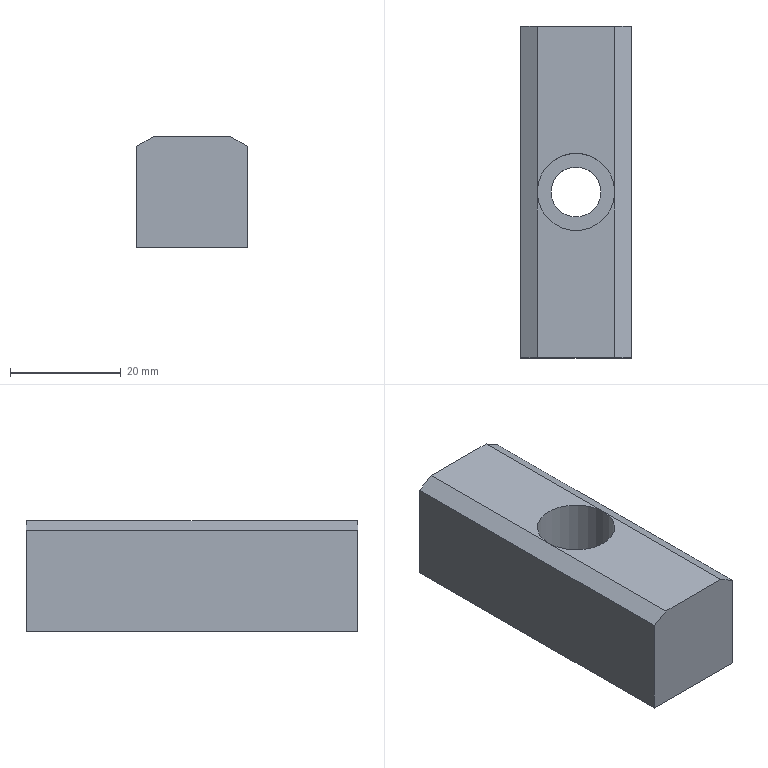Part | NX | features solid 2 | 1 solid | 12 faces | box 20 x 60 x 20 mm | volume 21513 mm3 | plane 10 | cylinder 2 | commonest cylinder face diameters 9 x1 14 x1
STEP:
#1=CARTESIAN_POINT('',(-7.,-353.,-45.));
#2=VERTEX_POINT('',#1);
#3=CARTESIAN_POINT('',(7.,-353.,-45.));
#4=VERTEX_POINT('',#3);
#5=CARTESIAN_POINT('',(-10.,-353.,-45.));
#6=DIRECTION('',(1.,0.,0.));
#7=VECTOR('',#6,1000.);
#8=LINE('',#5,#7);
#9=EDGE_CURVE('',#2,#4,#8,.T.);
#10=ORIENTED_EDGE('',*,*,#9,.T.);
#11=CARTESIAN_POINT('',(7.,-323.,-45.));
#12=VERTEX_POINT('',#11);
#13=CARTESIAN_POINT('',(7.,-353.,-45.));
#14=DIRECTION('',(0.,-1.,0.));
#15=VECTOR('',#14,1000.);
#16=LINE('',#13,#15);
#17=EDGE_CURVE('',#4,#12,#16,.F.);
#18=ORIENTED_EDGE('',*,*,#17,.T.);
#19=CARTESIAN_POINT('',(-7.,-323.,-45.));
#20=VERTEX_POINT('',#19);
#21=CARTESIAN_POINT('',(0.,-323.,-45.));
#22=DIRECTION('',(0.,0.,-1.));
#23=DIRECTION('',(-1.,0.,0.));
#24=AXIS2_PLACEMENT_3D('',#21,#22,#23);
#25=CIRCLE('',#24,7.);
#26=EDGE_CURVE('',#12,#20,#25,.T.);
#27=ORIENTED_EDGE('',*,*,#26,.T.);
#28=CARTESIAN_POINT('',(-7.,-353.,-45.));
#29=DIRECTION('',(0.,1.,0.));
#30=VECTOR('',#29,1000.);
#31=LINE('',#28,#30);
#32=EDGE_CURVE('',#20,#2,#31,.F.);
#33=ORIENTED_EDGE('',*,*,#32,.T.);
#34=EDGE_LOOP('',(#10,#18,#27,#33));
#35=FACE_BOUND('',#34,.T.);
#36=CARTESIAN_POINT('',(-10.,-353.,-45.));
#37=DIRECTION('',(0.,0.,-1.));
#38=DIRECTION('',(0.,1.,0.));
#39=AXIS2_PLACEMENT_3D('',#36,#37,#38);
#40=PLANE('',#39);
#41=ADVANCED_FACE('',(#35),#40,.F.);
#42=CARTESIAN_POINT('',(-4.5,-323.,-65.));
#43=VERTEX_POINT('',#42);
#44=CARTESIAN_POINT('',(0.,-323.,-65.));
#45=DIRECTION('',(0.,0.,-1.));
#46=DIRECTION('',(-1.,0.,0.));
#47=AXIS2_PLACEMENT_3D('',#44,#45,#46);
#48=CIRCLE('',#47,4.5);
#49=EDGE_CURVE('',#43,#43,#48,.T.);
#50=ORIENTED_EDGE('',*,*,#49,.F.);
#51=EDGE_LOOP('',(#50));
#52=FACE_BOUND('',#51,.T.);
#53=CARTESIAN_POINT('',(-10.,-353.,-65.));
#54=VERTEX_POINT('',#53);
#55=CARTESIAN_POINT('',(10.,-353.,-65.));
#56=VERTEX_POINT('',#55);
#57=CARTESIAN_POINT('',(-10.,-353.,-65.));
#58=DIRECTION('',(1.,0.,0.));
#59=VECTOR('',#58,1000.);
#60=LINE('',#57,#59);
#61=EDGE_CURVE('',#54,#56,#60,.T.);
#62=ORIENTED_EDGE('',*,*,#61,.F.);
#63=CARTESIAN_POINT('',(-10.,-293.,-65.));
#64=VERTEX_POINT('',#63);
#65=CARTESIAN_POINT('',(-10.,-353.,-65.));
#66=DIRECTION('',(0.,1.,0.));
#67=VECTOR('',#66,1000.);
#68=LINE('',#65,#67);
#69=EDGE_CURVE('',#54,#64,#68,.T.);
#70=ORIENTED_EDGE('',*,*,#69,.T.);
#71=CARTESIAN_POINT('',(10.,-293.,-65.));
#72=VERTEX_POINT('',#71);
#73=CARTESIAN_POINT('',(-10.,-293.,-65.));
#74=DIRECTION('',(1.,0.,0.));
#75=VECTOR('',#74,1000.);
#76=LINE('',#73,#75);
#77=EDGE_CURVE('',#64,#72,#76,.T.);
#78=ORIENTED_EDGE('',*,*,#77,.T.);
#79=CARTESIAN_POINT('',(10.,-353.,-65.));
#80=DIRECTION('',(0.,1.,0.));
#81=VECTOR('',#80,1000.);
#82=LINE('',#79,#81);
#83=EDGE_CURVE('',#56,#72,#82,.T.);
#84=ORIENTED_EDGE('',*,*,#83,.F.);
#85=EDGE_LOOP('',(#62,#70,#78,#84));
#86=FACE_BOUND('',#85,.T.);
#87=CARTESIAN_POINT('',(-10.,-353.,-65.));
#88=DIRECTION('',(0.,0.,-1.));
#89=DIRECTION('',(0.,1.,0.));
#90=AXIS2_PLACEMENT_3D('',#87,#88,#89);
#91=PLANE('',#90);
#92=ADVANCED_FACE('',(#52,#86),#91,.T.);
#93=CARTESIAN_POINT('',(-7.,-293.,-45.));
#94=VERTEX_POINT('',#93);
#95=CARTESIAN_POINT('',(7.,-293.,-45.));
#96=VERTEX_POINT('',#95);
#97=CARTESIAN_POINT('',(-10.,-293.,-45.));
#98=DIRECTION('',(1.,0.,0.));
#99=VECTOR('',#98,1000.);
#100=LINE('',#97,#99);
#101=EDGE_CURVE('',#94,#96,#100,.T.);
#102=ORIENTED_EDGE('',*,*,#101,.T.);
#103=CARTESIAN_POINT('',(10.,-293.,-46.732));
#104=VERTEX_POINT('',#103);
#105=CARTESIAN_POINT('',(2.91,-293.,-42.639));
#106=DIRECTION('',(0.866,0.,-0.5));
#107=VECTOR('',#106,1000.);
#108=LINE('',#105,#107);
#109=EDGE_CURVE('',#96,#104,#108,.T.);
#110=ORIENTED_EDGE('',*,*,#109,.T.);
#111=CARTESIAN_POINT('',(10.,-293.,-65.));
#112=DIRECTION('',(0.,0.,-1.));
#113=VECTOR('',#112,1000.);
#114=LINE('',#111,#113);
#115=EDGE_CURVE('',#72,#104,#114,.F.);
#116=ORIENTED_EDGE('',*,*,#115,.F.);
#117=ORIENTED_EDGE('',*,*,#77,.F.);
#118=CARTESIAN_POINT('',(-10.,-293.,-46.732));
#119=VERTEX_POINT('',#118);
#120=CARTESIAN_POINT('',(-10.,-293.,-65.));
#121=DIRECTION('',(0.,0.,1.));
#122=VECTOR('',#121,1000.);
#123=LINE('',#120,#122);
#124=EDGE_CURVE('',#64,#119,#123,.T.);
#125=ORIENTED_EDGE('',*,*,#124,.T.);
#126=CARTESIAN_POINT('',(-17.91,-293.,-51.299));
#127=DIRECTION('',(-0.866,0.,-0.5));
#128=VECTOR('',#127,1000.);
#129=LINE('',#126,#128);
#130=EDGE_CURVE('',#119,#94,#129,.F.);
#131=ORIENTED_EDGE('',*,*,#130,.T.);
#132=EDGE_LOOP('',(#102,#110,#116,#117,#125,#131));
#133=FACE_BOUND('',#132,.T.);
#134=CARTESIAN_POINT('',(-10.,-293.,-65.));
#135=DIRECTION('',(0.,1.,0.));
#136=DIRECTION('',(0.,0.,1.));
#137=AXIS2_PLACEMENT_3D('',#134,#135,#136);
#138=PLANE('',#137);
#139=ADVANCED_FACE('',(#133),#138,.T.);
#140=CARTESIAN_POINT('',(0.,-323.,-45.));
#141=DIRECTION('',(0.,0.,-1.));
#142=DIRECTION('',(-1.,0.,0.));
#143=AXIS2_PLACEMENT_3D('',#140,#141,#142);
#144=CIRCLE('',#143,7.);
#145=EDGE_CURVE('',#20,#12,#144,.T.);
#146=ORIENTED_EDGE('',*,*,#145,.T.);
#147=CARTESIAN_POINT('',(7.,-353.,-45.));
#148=DIRECTION('',(0.,-1.,0.));
#149=VECTOR('',#148,1000.);
#150=LINE('',#147,#149);
#151=EDGE_CURVE('',#12,#96,#150,.F.);
#152=ORIENTED_EDGE('',*,*,#151,.T.);
#153=ORIENTED_EDGE('',*,*,#101,.F.);
#154=CARTESIAN_POINT('',(-7.,-353.,-45.));
#155=DIRECTION('',(0.,1.,0.));
#156=VECTOR('',#155,1000.);
#157=LINE('',#154,#156);
#158=EDGE_CURVE('',#94,#20,#157,.F.);
#159=ORIENTED_EDGE('',*,*,#158,.T.);
#160=EDGE_LOOP('',(#146,#152,#153,#159));
#161=FACE_BOUND('',#160,.T.);
#162=CARTESIAN_POINT('',(-10.,-353.,-45.));
#163=DIRECTION('',(0.,0.,-1.));
#164=DIRECTION('',(0.,1.,0.));
#165=AXIS2_PLACEMENT_3D('',#162,#163,#164);
#166=PLANE('',#165);
#167=ADVANCED_FACE('',(#161),#166,.F.);
#168=ORIENTED_EDGE('',*,*,#115,.T.);
#169=CARTESIAN_POINT('',(10.,-353.,-46.732));
#170=VERTEX_POINT('',#169);
#171=CARTESIAN_POINT('',(10.,-353.,-46.732));
#172=DIRECTION('',(0.,-1.,0.));
#173=VECTOR('',#172,1000.);
#174=LINE('',#171,#173);
#175=EDGE_CURVE('',#104,#170,#174,.T.);
#176=ORIENTED_EDGE('',*,*,#175,.T.);
#177=CARTESIAN_POINT('',(10.,-353.,-65.));
#178=DIRECTION('',(0.,0.,-1.));
#179=VECTOR('',#178,1000.);
#180=LINE('',#177,#179);
#181=EDGE_CURVE('',#56,#170,#180,.F.);
#182=ORIENTED_EDGE('',*,*,#181,.F.);
#183=ORIENTED_EDGE('',*,*,#83,.T.);
#184=EDGE_LOOP('',(#168,#176,#182,#183));
#185=FACE_BOUND('',#184,.T.);
#186=CARTESIAN_POINT('',(10.,-353.,-65.));
#187=DIRECTION('',(1.,0.,0.));
#188=DIRECTION('',(0.,0.,-1.));
#189=AXIS2_PLACEMENT_3D('',#186,#187,#188);
#190=PLANE('',#189);
#191=ADVANCED_FACE('',(#185),#190,.T.);
#192=ORIENTED_EDGE('',*,*,#181,.T.);
#193=CARTESIAN_POINT('',(2.91,-353.,-42.639));
#194=DIRECTION('',(0.866,0.,-0.5));
#195=VECTOR('',#194,1000.);
#196=LINE('',#193,#195);
#197=EDGE_CURVE('',#170,#4,#196,.F.);
#198=ORIENTED_EDGE('',*,*,#197,.T.);
#199=ORIENTED_EDGE('',*,*,#9,.F.);
#200=CARTESIAN_POINT('',(-10.,-353.,-46.732));
#201=VERTEX_POINT('',#200);
#202=CARTESIAN_POINT('',(-17.91,-353.,-51.299));
#203=DIRECTION('',(-0.866,0.,-0.5));
#204=VECTOR('',#203,1000.);
#205=LINE('',#202,#204);
#206=EDGE_CURVE('',#2,#201,#205,.T.);
#207=ORIENTED_EDGE('',*,*,#206,.T.);
#208=CARTESIAN_POINT('',(-10.,-353.,-65.));
#209=DIRECTION('',(0.,0.,1.));
#210=VECTOR('',#209,1000.);
#211=LINE('',#208,#210);
#212=EDGE_CURVE('',#54,#201,#211,.T.);
#213=ORIENTED_EDGE('',*,*,#212,.F.);
#214=ORIENTED_EDGE('',*,*,#61,.T.);
#215=EDGE_LOOP('',(#192,#198,#199,#207,#213,#214));
#216=FACE_BOUND('',#215,.T.);
#217=CARTESIAN_POINT('',(-10.,-353.,-65.));
#218=DIRECTION('',(0.,1.,0.));
#219=DIRECTION('',(0.,0.,1.));
#220=AXIS2_PLACEMENT_3D('',#217,#218,#219);
#221=PLANE('',#220);
#222=ADVANCED_FACE('',(#216),#221,.F.);
#223=ORIENTED_EDGE('',*,*,#212,.T.);
#224=CARTESIAN_POINT('',(-10.,-293.,-46.732));
#225=DIRECTION('',(0.,1.,0.));
#226=VECTOR('',#225,1000.);
#227=LINE('',#224,#226);
#228=EDGE_CURVE('',#201,#119,#227,.T.);
#229=ORIENTED_EDGE('',*,*,#228,.T.);
#230=ORIENTED_EDGE('',*,*,#124,.F.);
#231=ORIENTED_EDGE('',*,*,#69,.F.);
#232=EDGE_LOOP('',(#223,#229,#230,#231));
#233=FACE_BOUND('',#232,.T.);
#234=CARTESIAN_POINT('',(-10.,-353.,-65.));
#235=DIRECTION('',(1.,0.,0.));
#236=DIRECTION('',(0.,0.,-1.));
#237=AXIS2_PLACEMENT_3D('',#234,#235,#236);
#238=PLANE('',#237);
#239=ADVANCED_FACE('',(#233),#238,.F.);
#240=ORIENTED_EDGE('',*,*,#49,.T.);
#241=EDGE_LOOP('',(#240));
#242=FACE_BOUND('',#241,.T.);
#243=CARTESIAN_POINT('',(-4.5,-323.,-55.));
#244=VERTEX_POINT('',#243);
#245=CARTESIAN_POINT('',(0.,-323.,-55.));
#246=DIRECTION('',(0.,0.,-1.));
#247=DIRECTION('',(-1.,0.,0.));
#248=AXIS2_PLACEMENT_3D('',#245,#246,#247);
#249=CIRCLE('',#248,4.5);
#250=EDGE_CURVE('',#244,#244,#249,.T.);
#251=ORIENTED_EDGE('',*,*,#250,.F.);
#252=EDGE_LOOP('',(#251));
#253=FACE_BOUND('',#252,.T.);
#254=CARTESIAN_POINT('',(0.,-323.,-95.));
#255=DIRECTION('',(0.,0.,-1.));
#256=DIRECTION('',(-1.,0.,0.));
#257=AXIS2_PLACEMENT_3D('',#254,#255,#256);
#258=CYLINDRICAL_SURFACE('',#257,4.5);
#259=ADVANCED_FACE('',(#242,#253),#258,.F.);
#260=ORIENTED_EDGE('',*,*,#250,.T.);
#261=EDGE_LOOP('',(#260));
#262=FACE_BOUND('',#261,.T.);
#263=CARTESIAN_POINT('',(-7.,-323.,-55.));
#264=VERTEX_POINT('',#263);
#265=CARTESIAN_POINT('',(0.,-323.,-55.));
#266=DIRECTION('',(0.,0.,-1.));
#267=DIRECTION('',(-1.,0.,0.));
#268=AXIS2_PLACEMENT_3D('',#265,#266,#267);
#269=CIRCLE('',#268,7.);
#270=EDGE_CURVE('',#264,#264,#269,.T.);
#271=ORIENTED_EDGE('',*,*,#270,.F.);
#272=EDGE_LOOP('',(#271));
#273=FACE_BOUND('',#272,.T.);
#274=CARTESIAN_POINT('',(0.,-323.,-55.));
#275=DIRECTION('',(0.,0.,-1.));
#276=DIRECTION('',(-1.,0.,0.));
#277=AXIS2_PLACEMENT_3D('',#274,#275,#276);
#278=PLANE('',#277);
#279=ADVANCED_FACE('',(#262,#273),#278,.F.);
#280=ORIENTED_EDGE('',*,*,#270,.T.);
#281=EDGE_LOOP('',(#280));
#282=FACE_BOUND('',#281,.T.);
#283=ORIENTED_EDGE('',*,*,#145,.F.);
#284=ORIENTED_EDGE('',*,*,#26,.F.);
#285=EDGE_LOOP('',(#283,#284));
#286=FACE_BOUND('',#285,.T.);
#287=CARTESIAN_POINT('',(0.,-323.,-45.));
#288=DIRECTION('',(0.,0.,-1.));
#289=DIRECTION('',(-1.,0.,0.));
#290=AXIS2_PLACEMENT_3D('',#287,#288,#289);
#291=CYLINDRICAL_SURFACE('',#290,7.);
#292=ADVANCED_FACE('',(#282,#286),#291,.F.);
#293=ORIENTED_EDGE('',*,*,#32,.F.);
#294=ORIENTED_EDGE('',*,*,#158,.F.);
#295=ORIENTED_EDGE('',*,*,#130,.F.);
#296=ORIENTED_EDGE('',*,*,#228,.F.);
#297=ORIENTED_EDGE('',*,*,#206,.F.);
#298=EDGE_LOOP('',(#293,#294,#295,#296,#297));
#299=FACE_BOUND('',#298,.T.);
#300=CARTESIAN_POINT('',(-10.,-353.,-46.732));
#301=DIRECTION('',(0.5,0.,-0.866));
#302=DIRECTION('',(-0.866,0.,-0.5));
#303=AXIS2_PLACEMENT_3D('',#300,#301,#302);
#304=PLANE('',#303);
#305=ADVANCED_FACE('',(#299),#304,.F.);
#306=ORIENTED_EDGE('',*,*,#197,.F.);
#307=ORIENTED_EDGE('',*,*,#175,.F.);
#308=ORIENTED_EDGE('',*,*,#109,.F.);
#309=ORIENTED_EDGE('',*,*,#151,.F.);
#310=ORIENTED_EDGE('',*,*,#17,.F.);
#311=EDGE_LOOP('',(#306,#307,#308,#309,#310));
#312=FACE_BOUND('',#311,.T.);
#313=CARTESIAN_POINT('',(7.,-353.,-45.));
#314=DIRECTION('',(0.5,0.,0.866));
#315=DIRECTION('',(0.866,0.,-0.5));
#316=AXIS2_PLACEMENT_3D('',#313,#314,#315);
#317=PLANE('',#316);
#318=ADVANCED_FACE('',(#312),#317,.T.);
#319=CLOSED_SHELL('',(#41,#92,#139,#167,#191,#222,#239,#259,#279,#292,#305,#318));
#320=MANIFOLD_SOLID_BREP('',#319);
#321=(LENGTH_UNIT()NAMED_UNIT(*)SI_UNIT(.MILLI.,.METRE.));
#322=UNCERTAINTY_MEASURE_WITH_UNIT(LENGTH_MEASURE(0.00001),#321,'','');
#323=(NAMED_UNIT(*)PLANE_ANGLE_UNIT()SI_UNIT($,.RADIAN.));
#324=(NAMED_UNIT(*)SI_UNIT($,.STERADIAN.)SOLID_ANGLE_UNIT());
#325=(GEOMETRIC_REPRESENTATION_CONTEXT(3)GLOBAL_UNCERTAINTY_ASSIGNED_CONTEXT((#322))GLOBAL_UNIT_ASSIGNED_CONTEXT((#321,#323,#324))REPRESENTATION_CONTEXT('',''));
#326=ADVANCED_BREP_SHAPE_REPRESENTATION('',(#320),#325);